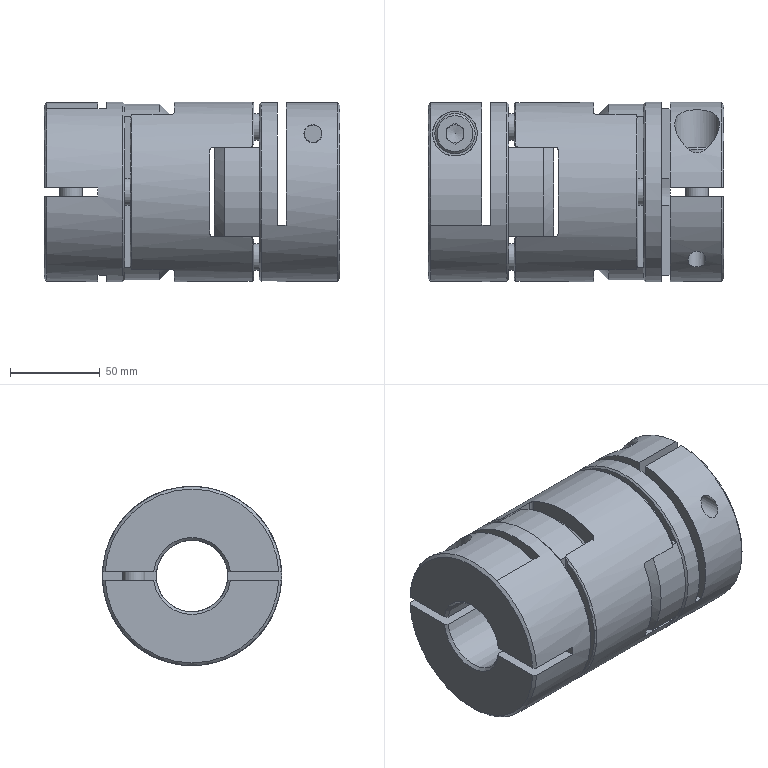Part | NX | features BREP 5 | 5 solids | 140 faces | box 165 x 100 x 100 mm | volume 960558 mm3 | plane 80 | cylinder 36 | cone 20 | torus 4 | commonest cylinder face diameters 100 x5 3 x4 5 x4 15 x4 40 x4 98 x4